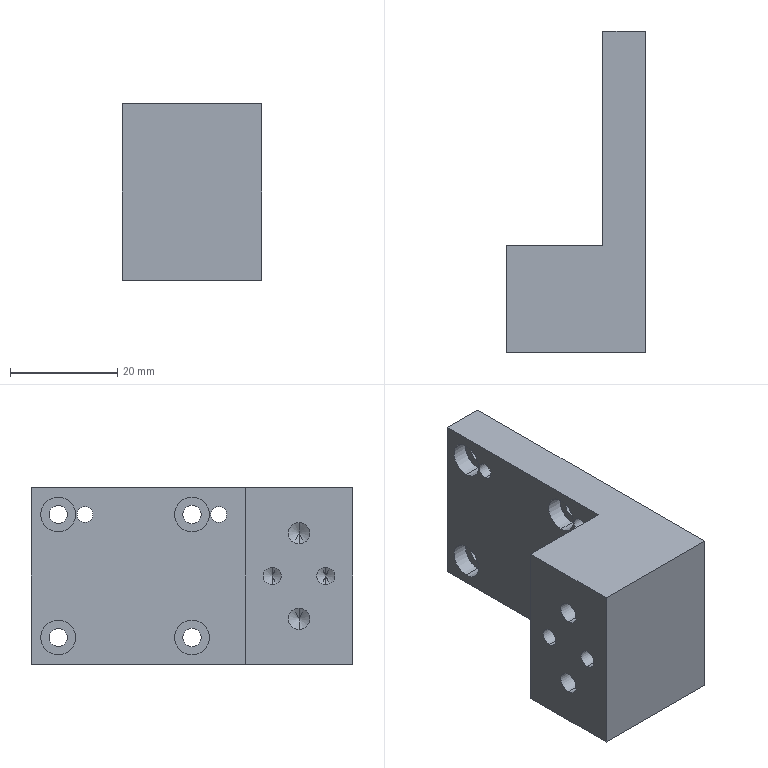Part | SolidWorks | features HoleWzd 4, LPattern 4, ICE 2, Extrusion 1 | 1 solid | 48 faces | box 26 x 60 x 33 mm | volume 26587 mm3 | cylinder 28 | plane 12 | cone 8 | commonest cylinder face diameters 3.4 x8 6.5 x8 3 x4 3.3 x4 4 x4
STEP:
#1=CARTESIAN_POINT('',(-8.,-20.,6.));
#2=VERTEX_POINT('',#1);
#3=CARTESIAN_POINT('',(-8.,-20.,10.));
#4=VERTEX_POINT('',#3);
#5=CARTESIAN_POINT('',(-8.,-20.,8.));
#6=DIRECTION('',(-1.,0.,0.));
#7=DIRECTION('',(0.,0.,1.));
#8=AXIS2_PLACEMENT_3D('',#5,#6,#7);
#9=CIRCLE('',#8,2.);
#10=EDGE_CURVE('',#2,#4,#9,.T.);
#11=ORIENTED_EDGE('',*,*,#10,.F.);
#12=CARTESIAN_POINT('',(-18.,-20.,6.));
#13=VERTEX_POINT('',#12);
#14=CARTESIAN_POINT('',(-18.,-20.,6.));
#15=DIRECTION('',(-1.,0.,0.));
#16=VECTOR('',#15,1000.);
#17=LINE('',#14,#16);
#18=EDGE_CURVE('',#2,#13,#17,.T.);
#19=ORIENTED_EDGE('',*,*,#18,.T.);
#20=CARTESIAN_POINT('',(-18.,-20.,10.));
#21=VERTEX_POINT('',#20);
#22=CARTESIAN_POINT('',(-18.,-20.,8.));
#23=DIRECTION('',(-1.,0.,0.));
#24=DIRECTION('',(0.,0.,1.));
#25=AXIS2_PLACEMENT_3D('',#22,#23,#24);
#26=CIRCLE('',#25,2.);
#27=EDGE_CURVE('',#13,#21,#26,.T.);
#28=ORIENTED_EDGE('',*,*,#27,.T.);
#29=CARTESIAN_POINT('',(-18.,-20.,10.));
#30=DIRECTION('',(-1.,0.,0.));
#31=VECTOR('',#30,1000.);
#32=LINE('',#29,#31);
#33=EDGE_CURVE('',#4,#21,#32,.T.);
#34=ORIENTED_EDGE('',*,*,#33,.F.);
#35=EDGE_LOOP('',(#11,#19,#28,#34));
#36=FACE_OUTER_BOUND('',#35,.T.);
#37=CARTESIAN_POINT('',(-18.,-20.,8.));
#38=DIRECTION('',(-1.,0.,0.));
#39=DIRECTION('',(0.,0.,1.));
#40=AXIS2_PLACEMENT_3D('',#37,#38,#39);
#41=CYLINDRICAL_SURFACE('',#40,2.);
#42=ADVANCED_FACE('',(#36),#41,.F.);
#43=CARTESIAN_POINT('',(-6.798,-20.,8.));
#44=VERTEX_POINT('',#43);
#45=CARTESIAN_POINT('',(-8.,-20.,10.));
#46=DIRECTION('',(-0.515,0.,0.8572));
#47=VECTOR('',#46,1000.);
#48=LINE('',#45,#47);
#49=EDGE_CURVE('',#44,#4,#48,.T.);
#50=ORIENTED_EDGE('',*,*,#49,.F.);
#51=CARTESIAN_POINT('',(-8.,-20.,6.));
#52=DIRECTION('',(-0.515,0.,-0.8572));
#53=VECTOR('',#52,1000.);
#54=LINE('',#51,#53);
#55=EDGE_CURVE('',#44,#2,#54,.T.);
#56=ORIENTED_EDGE('',*,*,#55,.T.);
#57=ORIENTED_EDGE('',*,*,#10,.T.);
#58=EDGE_LOOP('',(#50,#56,#57));
#59=FACE_OUTER_BOUND('',#58,.T.);
#60=CARTESIAN_POINT('',(-8.,-20.,8.));
#61=DIRECTION('',(-1.,0.,0.));
#62=DIRECTION('',(0.,0.,1.));
#63=AXIS2_PLACEMENT_3D('',#60,#61,#62);
#64=CONICAL_SURFACE('',#63,2.,1.03);
#65=ADVANCED_FACE('',(#59),#64,.F.);
#66=CARTESIAN_POINT('',(-8.,-20.,-10.));
#67=VERTEX_POINT('',#66);
#68=CARTESIAN_POINT('',(-8.,-20.,-6.));
#69=VERTEX_POINT('',#68);
#70=CARTESIAN_POINT('',(-8.,-20.,-8.));
#71=DIRECTION('',(-1.,0.,0.));
#72=DIRECTION('',(0.,0.,1.));
#73=AXIS2_PLACEMENT_3D('',#70,#71,#72);
#74=CIRCLE('',#73,2.);
#75=EDGE_CURVE('',#67,#69,#74,.T.);
#76=ORIENTED_EDGE('',*,*,#75,.F.);
#77=CARTESIAN_POINT('',(-18.,-20.,-10.));
#78=VERTEX_POINT('',#77);
#79=CARTESIAN_POINT('',(-18.,-20.,-10.));
#80=DIRECTION('',(-1.,0.,0.));
#81=VECTOR('',#80,1000.);
#82=LINE('',#79,#81);
#83=EDGE_CURVE('',#67,#78,#82,.T.);
#84=ORIENTED_EDGE('',*,*,#83,.T.);
#85=CARTESIAN_POINT('',(-18.,-20.,-6.));
#86=VERTEX_POINT('',#85);
#87=CARTESIAN_POINT('',(-18.,-20.,-8.));
#88=DIRECTION('',(-1.,0.,0.));
#89=DIRECTION('',(0.,0.,1.));
#90=AXIS2_PLACEMENT_3D('',#87,#88,#89);
#91=CIRCLE('',#90,2.);
#92=EDGE_CURVE('',#78,#86,#91,.T.);
#93=ORIENTED_EDGE('',*,*,#92,.T.);
#94=CARTESIAN_POINT('',(-18.,-20.,-6.));
#95=DIRECTION('',(-1.,0.,0.));
#96=VECTOR('',#95,1000.);
#97=LINE('',#94,#96);
#98=EDGE_CURVE('',#69,#86,#97,.T.);
#99=ORIENTED_EDGE('',*,*,#98,.F.);
#100=EDGE_LOOP('',(#76,#84,#93,#99));
#101=FACE_OUTER_BOUND('',#100,.T.);
#102=CARTESIAN_POINT('',(-18.,-20.,-8.));
#103=DIRECTION('',(-1.,0.,0.));
#104=DIRECTION('',(0.,0.,1.));
#105=AXIS2_PLACEMENT_3D('',#102,#103,#104);
#106=CYLINDRICAL_SURFACE('',#105,2.);
#107=ADVANCED_FACE('',(#101),#106,.F.);
#108=CARTESIAN_POINT('',(-6.798,-20.,-8.));
#109=VERTEX_POINT('',#108);
#110=CARTESIAN_POINT('',(-8.,-20.,-6.));
#111=DIRECTION('',(-0.515,0.,0.8572));
#112=VECTOR('',#111,1000.);
#113=LINE('',#110,#112);
#114=EDGE_CURVE('',#109,#69,#113,.T.);
#115=ORIENTED_EDGE('',*,*,#114,.F.);
#116=CARTESIAN_POINT('',(-8.,-20.,-10.));
#117=DIRECTION('',(-0.515,0.,-0.8572));
#118=VECTOR('',#117,1000.);
#119=LINE('',#116,#118);
#120=EDGE_CURVE('',#109,#67,#119,.T.);
#121=ORIENTED_EDGE('',*,*,#120,.T.);
#122=ORIENTED_EDGE('',*,*,#75,.T.);
#123=EDGE_LOOP('',(#115,#121,#122));
#124=FACE_OUTER_BOUND('',#123,.T.);
#125=CARTESIAN_POINT('',(-8.,-20.,-8.));
#126=DIRECTION('',(-1.,0.,0.));
#127=DIRECTION('',(0.,0.,1.));
#128=AXIS2_PLACEMENT_3D('',#125,#126,#127);
#129=CONICAL_SURFACE('',#128,2.,1.03);
#130=ADVANCED_FACE('',(#124),#129,.F.);
#131=CARTESIAN_POINT('',(8.,-5.,10.));
#132=VERTEX_POINT('',#131);
#133=CARTESIAN_POINT('',(8.,-5.,13.));
#134=VERTEX_POINT('',#133);
#135=CARTESIAN_POINT('',(8.,-5.,11.5));
#136=DIRECTION('',(-1.,0.,0.));
#137=DIRECTION('',(0.,0.,1.));
#138=AXIS2_PLACEMENT_3D('',#135,#136,#137);
#139=CIRCLE('',#138,1.5);
#140=EDGE_CURVE('',#132,#134,#139,.T.);
#141=ORIENTED_EDGE('',*,*,#140,.F.);
#142=CARTESIAN_POINT('',(0.,-5.,10.));
#143=VERTEX_POINT('',#142);
#144=CARTESIAN_POINT('',(0.,-5.,10.));
#145=DIRECTION('',(-1.,0.,0.));
#146=VECTOR('',#145,1000.);
#147=LINE('',#144,#146);
#148=EDGE_CURVE('',#132,#143,#147,.T.);
#149=ORIENTED_EDGE('',*,*,#148,.T.);
#150=CARTESIAN_POINT('',(0.,-5.,13.));
#151=VERTEX_POINT('',#150);
#152=CARTESIAN_POINT('',(0.,-5.,11.5));
#153=DIRECTION('',(-1.,0.,0.));
#154=DIRECTION('',(0.,0.,1.));
#155=AXIS2_PLACEMENT_3D('',#152,#153,#154);
#156=CIRCLE('',#155,1.5);
#157=EDGE_CURVE('',#143,#151,#156,.T.);
#158=ORIENTED_EDGE('',*,*,#157,.T.);
#159=CARTESIAN_POINT('',(0.,-5.,13.));
#160=DIRECTION('',(-1.,0.,0.));
#161=VECTOR('',#160,1000.);
#162=LINE('',#159,#161);
#163=EDGE_CURVE('',#134,#151,#162,.T.);
#164=ORIENTED_EDGE('',*,*,#163,.F.);
#165=EDGE_LOOP('',(#141,#149,#158,#164));
#166=FACE_OUTER_BOUND('',#165,.T.);
#167=CARTESIAN_POINT('',(0.,-5.,11.5));
#168=DIRECTION('',(-1.,0.,0.));
#169=DIRECTION('',(0.,0.,1.));
#170=AXIS2_PLACEMENT_3D('',#167,#168,#169);
#171=CYLINDRICAL_SURFACE('',#170,1.5);
#172=ADVANCED_FACE('',(#166),#171,.F.);
#173=CARTESIAN_POINT('',(8.,20.,10.));
#174=VERTEX_POINT('',#173);
#175=CARTESIAN_POINT('',(8.,20.,13.));
#176=VERTEX_POINT('',#175);
#177=CARTESIAN_POINT('',(8.,20.,11.5));
#178=DIRECTION('',(-1.,0.,0.));
#179=DIRECTION('',(0.,0.,1.));
#180=AXIS2_PLACEMENT_3D('',#177,#178,#179);
#181=CIRCLE('',#180,1.5);
#182=EDGE_CURVE('',#174,#176,#181,.T.);
#183=ORIENTED_EDGE('',*,*,#182,.F.);
#184=CARTESIAN_POINT('',(0.,20.,10.));
#185=VERTEX_POINT('',#184);
#186=CARTESIAN_POINT('',(0.,20.,10.));
#187=DIRECTION('',(-1.,0.,0.));
#188=VECTOR('',#187,1000.);
#189=LINE('',#186,#188);
#190=EDGE_CURVE('',#174,#185,#189,.T.);
#191=ORIENTED_EDGE('',*,*,#190,.T.);
#192=CARTESIAN_POINT('',(0.,20.,13.));
#193=VERTEX_POINT('',#192);
#194=CARTESIAN_POINT('',(0.,20.,11.5));
#195=DIRECTION('',(-1.,0.,0.));
#196=DIRECTION('',(0.,0.,1.));
#197=AXIS2_PLACEMENT_3D('',#194,#195,#196);
#198=CIRCLE('',#197,1.5);
#199=EDGE_CURVE('',#185,#193,#198,.T.);
#200=ORIENTED_EDGE('',*,*,#199,.T.);
#201=CARTESIAN_POINT('',(0.,20.,13.));
#202=DIRECTION('',(-1.,0.,0.));
#203=VECTOR('',#202,1000.);
#204=LINE('',#201,#203);
#205=EDGE_CURVE('',#176,#193,#204,.T.);
#206=ORIENTED_EDGE('',*,*,#205,.F.);
#207=EDGE_LOOP('',(#183,#191,#200,#206));
#208=FACE_OUTER_BOUND('',#207,.T.);
#209=CARTESIAN_POINT('',(0.,20.,11.5));
#210=DIRECTION('',(-1.,0.,0.));
#211=DIRECTION('',(0.,0.,1.));
#212=AXIS2_PLACEMENT_3D('',#209,#210,#211);
#213=CYLINDRICAL_SURFACE('',#212,1.5);
#214=ADVANCED_FACE('',(#208),#213,.F.);
#215=CARTESIAN_POINT('',(-7.9,-15.,-1.65));
#216=VERTEX_POINT('',#215);
#217=CARTESIAN_POINT('',(-7.9,-15.,1.65));
#218=VERTEX_POINT('',#217);
#219=CARTESIAN_POINT('',(-7.9,-15.,0.));
#220=DIRECTION('',(-1.,0.,0.));
#221=DIRECTION('',(0.,0.,1.));
#222=AXIS2_PLACEMENT_3D('',#219,#220,#221);
#223=CIRCLE('',#222,1.65);
#224=EDGE_CURVE('',#216,#218,#223,.T.);
#225=ORIENTED_EDGE('',*,*,#224,.F.);
#226=CARTESIAN_POINT('',(-18.,-15.,-1.65));
#227=VERTEX_POINT('',#226);
#228=CARTESIAN_POINT('',(-18.,-15.,-1.65));
#229=DIRECTION('',(-1.,0.,0.));
#230=VECTOR('',#229,1000.);
#231=LINE('',#228,#230);
#232=EDGE_CURVE('',#216,#227,#231,.T.);
#233=ORIENTED_EDGE('',*,*,#232,.T.);
#234=CARTESIAN_POINT('',(-18.,-15.,1.65));
#235=VERTEX_POINT('',#234);
#236=CARTESIAN_POINT('',(-18.,-15.,0.));
#237=DIRECTION('',(-1.,0.,0.));
#238=DIRECTION('',(0.,0.,1.));
#239=AXIS2_PLACEMENT_3D('',#236,#237,#238);
#240=CIRCLE('',#239,1.65);
#241=EDGE_CURVE('',#227,#235,#240,.T.);
#242=ORIENTED_EDGE('',*,*,#241,.T.);
#243=CARTESIAN_POINT('',(-18.,-15.,1.65));
#244=DIRECTION('',(-1.,0.,0.));
#245=VECTOR('',#244,1000.);
#246=LINE('',#243,#245);
#247=EDGE_CURVE('',#218,#235,#246,.T.);
#248=ORIENTED_EDGE('',*,*,#247,.F.);
#249=EDGE_LOOP('',(#225,#233,#242,#248));
#250=FACE_OUTER_BOUND('',#249,.T.);
#251=CARTESIAN_POINT('',(-18.,-15.,0.));
#252=DIRECTION('',(-1.,0.,0.));
#253=DIRECTION('',(0.,0.,1.));
#254=AXIS2_PLACEMENT_3D('',#251,#252,#253);
#255=CYLINDRICAL_SURFACE('',#254,1.65);
#256=ADVANCED_FACE('',(#250),#255,.F.);
#257=CARTESIAN_POINT('',(-6.909,-15.,0.));
#258=VERTEX_POINT('',#257);
#259=CARTESIAN_POINT('',(-7.9,-15.,1.65));
#260=DIRECTION('',(-0.515,0.,0.8572));
#261=VECTOR('',#260,1000.);
#262=LINE('',#259,#261);
#263=EDGE_CURVE('',#258,#218,#262,.T.);
#264=ORIENTED_EDGE('',*,*,#263,.F.);
#265=CARTESIAN_POINT('',(-7.9,-15.,-1.65));
#266=DIRECTION('',(-0.515,0.,-0.8572));
#267=VECTOR('',#266,1000.);
#268=LINE('',#265,#267);
#269=EDGE_CURVE('',#258,#216,#268,.T.);
#270=ORIENTED_EDGE('',*,*,#269,.T.);
#271=ORIENTED_EDGE('',*,*,#224,.T.);
#272=EDGE_LOOP('',(#264,#270,#271));
#273=FACE_OUTER_BOUND('',#272,.T.);
#274=CARTESIAN_POINT('',(-7.9,-15.,0.));
#275=DIRECTION('',(-1.,0.,0.));
#276=DIRECTION('',(0.,0.,1.));
#277=AXIS2_PLACEMENT_3D('',#274,#275,#276);
#278=CONICAL_SURFACE('',#277,1.65,1.03);
#279=ADVANCED_FACE('',(#273),#278,.F.);
#280=CARTESIAN_POINT('',(-7.9,-25.,-1.65));
#281=VERTEX_POINT('',#280);
#282=CARTESIAN_POINT('',(-7.9,-25.,1.65));
#283=VERTEX_POINT('',#282);
#284=CARTESIAN_POINT('',(-7.9,-25.,0.));
#285=DIRECTION('',(-1.,0.,0.));
#286=DIRECTION('',(0.,0.,1.));
#287=AXIS2_PLACEMENT_3D('',#284,#285,#286);
#288=CIRCLE('',#287,1.65);
#289=EDGE_CURVE('',#281,#283,#288,.T.);
#290=ORIENTED_EDGE('',*,*,#289,.F.);
#291=CARTESIAN_POINT('',(-18.,-25.,-1.65));
#292=VERTEX_POINT('',#291);
#293=CARTESIAN_POINT('',(-18.,-25.,-1.65));
#294=DIRECTION('',(-1.,0.,0.));
#295=VECTOR('',#294,1000.);
#296=LINE('',#293,#295);
#297=EDGE_CURVE('',#281,#292,#296,.T.);
#298=ORIENTED_EDGE('',*,*,#297,.T.);
#299=CARTESIAN_POINT('',(-18.,-25.,1.65));
#300=VERTEX_POINT('',#299);
#301=CARTESIAN_POINT('',(-18.,-25.,0.));
#302=DIRECTION('',(-1.,0.,0.));
#303=DIRECTION('',(0.,0.,1.));
#304=AXIS2_PLACEMENT_3D('',#301,#302,#303);
#305=CIRCLE('',#304,1.65);
#306=EDGE_CURVE('',#292,#300,#305,.T.);
#307=ORIENTED_EDGE('',*,*,#306,.T.);
#308=CARTESIAN_POINT('',(-18.,-25.,1.65));
#309=DIRECTION('',(-1.,0.,0.));
#310=VECTOR('',#309,1000.);
#311=LINE('',#308,#310);
#312=EDGE_CURVE('',#283,#300,#311,.T.);
#313=ORIENTED_EDGE('',*,*,#312,.F.);
#314=EDGE_LOOP('',(#290,#298,#307,#313));
#315=FACE_OUTER_BOUND('',#314,.T.);
#316=CARTESIAN_POINT('',(-18.,-25.,0.));
#317=DIRECTION('',(-1.,0.,0.));
#318=DIRECTION('',(0.,0.,1.));
#319=AXIS2_PLACEMENT_3D('',#316,#317,#318);
#320=CYLINDRICAL_SURFACE('',#319,1.65);
#321=ADVANCED_FACE('',(#315),#320,.F.);
#322=CARTESIAN_POINT('',(-6.909,-25.,0.));
#323=VERTEX_POINT('',#322);
#324=CARTESIAN_POINT('',(-7.9,-25.,1.65));
#325=DIRECTION('',(-0.515,0.,0.8572));
#326=VECTOR('',#325,1000.);
#327=LINE('',#324,#326);
#328=EDGE_CURVE('',#323,#283,#327,.T.);
#329=ORIENTED_EDGE('',*,*,#328,.F.);
#330=CARTESIAN_POINT('',(-7.9,-25.,-1.65));
#331=DIRECTION('',(-0.515,0.,-0.8572));
#332=VECTOR('',#331,1000.);
#333=LINE('',#330,#332);
#334=EDGE_CURVE('',#323,#281,#333,.T.);
#335=ORIENTED_EDGE('',*,*,#334,.T.);
#336=ORIENTED_EDGE('',*,*,#289,.T.);
#337=EDGE_LOOP('',(#329,#335,#336));
#338=FACE_OUTER_BOUND('',#337,.T.);
#339=CARTESIAN_POINT('',(-7.9,-25.,0.));
#340=DIRECTION('',(-1.,0.,0.));
#341=DIRECTION('',(0.,0.,1.));
#342=AXIS2_PLACEMENT_3D('',#339,#340,#341);
#343=CONICAL_SURFACE('',#342,1.65,1.03);
#344=ADVANCED_FACE('',(#338),#343,.F.);
#345=CARTESIAN_POINT('',(8.,0.,9.8));
#346=VERTEX_POINT('',#345);
#347=CARTESIAN_POINT('',(8.,0.,13.2));
#348=VERTEX_POINT('',#347);
#349=CARTESIAN_POINT('',(8.,0.,11.5));
#350=DIRECTION('',(-1.,0.,0.));
#351=DIRECTION('',(0.,0.,1.));
#352=AXIS2_PLACEMENT_3D('',#349,#350,#351);
#353=CIRCLE('',#352,1.7);
#354=EDGE_CURVE('',#346,#348,#353,.T.);
#355=ORIENTED_EDGE('',*,*,#354,.F.);
#356=CARTESIAN_POINT('',(3.,0.,9.8));
#357=VERTEX_POINT('',#356);
#358=CARTESIAN_POINT('',(0.,0.,9.8));
#359=DIRECTION('',(-1.,0.,0.));
#360=VECTOR('',#359,1000.);
#361=LINE('',#358,#360);
#362=EDGE_CURVE('',#346,#357,#361,.T.);
#363=ORIENTED_EDGE('',*,*,#362,.T.);
#364=CARTESIAN_POINT('',(3.,0.,13.2));
#365=VERTEX_POINT('',#364);
#366=CARTESIAN_POINT('',(3.,0.,11.5));
#367=DIRECTION('',(-1.,0.,0.));
#368=DIRECTION('',(0.,0.,1.));
#369=AXIS2_PLACEMENT_3D('',#366,#367,#368);
#370=CIRCLE('',#369,1.7);
#371=EDGE_CURVE('',#357,#365,#370,.T.);
#372=ORIENTED_EDGE('',*,*,#371,.T.);
#373=CARTESIAN_POINT('',(0.,0.,13.2));
#374=DIRECTION('',(-1.,0.,0.));
#375=VECTOR('',#374,1000.);
#376=LINE('',#373,#375);
#377=EDGE_CURVE('',#348,#365,#376,.T.);
#378=ORIENTED_EDGE('',*,*,#377,.F.);
#379=EDGE_LOOP('',(#355,#363,#372,#378));
#380=FACE_OUTER_BOUND('',#379,.T.);
#381=CARTESIAN_POINT('',(0.,0.,11.5));
#382=DIRECTION('',(-1.,0.,0.));
#383=DIRECTION('',(0.,0.,1.));
#384=AXIS2_PLACEMENT_3D('',#381,#382,#383);
#385=CYLINDRICAL_SURFACE('',#384,1.7);
#386=ADVANCED_FACE('',(#380),#385,.F.);
#387=CARTESIAN_POINT('',(3.,0.,8.25));
#388=VERTEX_POINT('',#387);
#389=CARTESIAN_POINT('',(3.,0.,14.75));
#390=VERTEX_POINT('',#389);
#391=CARTESIAN_POINT('',(3.,0.,11.5));
#392=DIRECTION('',(-1.,0.,0.));
#393=DIRECTION('',(0.,0.,1.));
#394=AXIS2_PLACEMENT_3D('',#391,#392,#393);
#395=CIRCLE('',#394,3.25);
#396=EDGE_CURVE('',#388,#390,#395,.T.);
#397=ORIENTED_EDGE('',*,*,#396,.F.);
#398=CARTESIAN_POINT('',(0.,0.,8.25));
#399=VERTEX_POINT('',#398);
#400=CARTESIAN_POINT('',(0.,0.,8.25));
#401=DIRECTION('',(-1.,0.,0.));
#402=VECTOR('',#401,1000.);
#403=LINE('',#400,#402);
#404=EDGE_CURVE('',#388,#399,#403,.T.);
#405=ORIENTED_EDGE('',*,*,#404,.T.);
#406=CARTESIAN_POINT('',(0.,0.,14.75));
#407=VERTEX_POINT('',#406);
#408=CARTESIAN_POINT('',(0.,0.,11.5));
#409=DIRECTION('',(-1.,0.,0.));
#410=DIRECTION('',(0.,0.,1.));
#411=AXIS2_PLACEMENT_3D('',#408,#409,#410);
#412=CIRCLE('',#411,3.25);
#413=EDGE_CURVE('',#399,#407,#412,.T.);
#414=ORIENTED_EDGE('',*,*,#413,.T.);
#415=CARTESIAN_POINT('',(0.,0.,14.75));
#416=DIRECTION('',(-1.,0.,0.));
#417=VECTOR('',#416,1000.);
#418=LINE('',#415,#417);
#419=EDGE_CURVE('',#390,#407,#418,.T.);
#420=ORIENTED_EDGE('',*,*,#419,.F.);
#421=EDGE_LOOP('',(#397,#405,#414,#420));
#422=FACE_OUTER_BOUND('',#421,.T.);
#423=CARTESIAN_POINT('',(0.,0.,11.5));
#424=DIRECTION('',(-1.,0.,0.));
#425=DIRECTION('',(0.,0.,1.));
#426=AXIS2_PLACEMENT_3D('',#423,#424,#425);
#427=CYLINDRICAL_SURFACE('',#426,3.25);
#428=ADVANCED_FACE('',(#422),#427,.F.);
#429=CARTESIAN_POINT('',(8.,0.,-13.2));
#430=VERTEX_POINT('',#429);
#431=CARTESIAN_POINT('',(8.,0.,-9.8));
#432=VERTEX_POINT('',#431);
#433=CARTESIAN_POINT('',(8.,0.,-11.5));
#434=DIRECTION('',(-1.,0.,0.));
#435=DIRECTION('',(0.,0.,1.));
#436=AXIS2_PLACEMENT_3D('',#433,#434,#435);
#437=CIRCLE('',#436,1.7);
#438=EDGE_CURVE('',#430,#432,#437,.T.);
#439=ORIENTED_EDGE('',*,*,#438,.F.);
#440=CARTESIAN_POINT('',(3.,0.,-13.2));
#441=VERTEX_POINT('',#440);
#442=CARTESIAN_POINT('',(0.,0.,-13.2));
#443=DIRECTION('',(-1.,0.,0.));
#444=VECTOR('',#443,1000.);
#445=LINE('',#442,#444);
#446=EDGE_CURVE('',#430,#441,#445,.T.);
#447=ORIENTED_EDGE('',*,*,#446,.T.);
#448=CARTESIAN_POINT('',(3.,0.,-9.8));
#449=VERTEX_POINT('',#448);
#450=CARTESIAN_POINT('',(3.,0.,-11.5));
#451=DIRECTION('',(-1.,0.,0.));
#452=DIRECTION('',(0.,0.,1.));
#453=AXIS2_PLACEMENT_3D('',#450,#451,#452);
#454=CIRCLE('',#453,1.7);
#455=EDGE_CURVE('',#441,#449,#454,.T.);
#456=ORIENTED_EDGE('',*,*,#455,.T.);
#457=CARTESIAN_POINT('',(0.,0.,-9.8));
#458=DIRECTION('',(-1.,0.,0.));
#459=VECTOR('',#458,1000.);
#460=LINE('',#457,#459);
#461=EDGE_CURVE('',#432,#449,#460,.T.);
#462=ORIENTED_EDGE('',*,*,#461,.F.);
#463=EDGE_LOOP('',(#439,#447,#456,#462));
#464=FACE_OUTER_BOUND('',#463,.T.);
#465=CARTESIAN_POINT('',(0.,0.,-11.5));
#466=DIRECTION('',(-1.,0.,0.));
#467=DIRECTION('',(0.,0.,1.));
#468=AXIS2_PLACEMENT_3D('',#465,#466,#467);
#469=CYLINDRICAL_SURFACE('',#468,1.7);
#470=ADVANCED_FACE('',(#464),#469,.F.);
#471=CARTESIAN_POINT('',(3.,0.,-14.75));
#472=VERTEX_POINT('',#471);
#473=CARTESIAN_POINT('',(3.,0.,-8.25));
#474=VERTEX_POINT('',#473);
#475=CARTESIAN_POINT('',(3.,0.,-11.5));
#476=DIRECTION('',(-1.,0.,0.));
#477=DIRECTION('',(0.,0.,1.));
#478=AXIS2_PLACEMENT_3D('',#475,#476,#477);
#479=CIRCLE('',#478,3.25);
#480=EDGE_CURVE('',#472,#474,#479,.T.);
#481=ORIENTED_EDGE('',*,*,#480,.F.);
#482=CARTESIAN_POINT('',(0.,0.,-14.75));
#483=VERTEX_POINT('',#482);
#484=CARTESIAN_POINT('',(0.,0.,-14.75));
#485=DIRECTION('',(-1.,0.,0.));
#486=VECTOR('',#485,1000.);
#487=LINE('',#484,#486);
#488=EDGE_CURVE('',#472,#483,#487,.T.);
#489=ORIENTED_EDGE('',*,*,#488,.T.);
#490=CARTESIAN_POINT('',(0.,0.,-8.25));
#491=VERTEX_POINT('',#490);
#492=CARTESIAN_POINT('',(0.,0.,-11.5));
#493=DIRECTION('',(-1.,0.,0.));
#494=DIRECTION('',(0.,0.,1.));
#495=AXIS2_PLACEMENT_3D('',#492,#493,#494);
#496=CIRCLE('',#495,3.25);
#497=EDGE_CURVE('',#483,#491,#496,.T.);
#498=ORIENTED_EDGE('',*,*,#497,.T.);
#499=CARTESIAN_POINT('',(0.,0.,-8.25));
#500=DIRECTION('',(-1.,0.,0.));
#501=VECTOR('',#500,1000.);
#502=LINE('',#499,#501);
#503=EDGE_CURVE('',#474,#491,#502,.T.);
#504=ORIENTED_EDGE('',*,*,#503,.F.);
#505=EDGE_LOOP('',(#481,#489,#498,#504));
#506=FACE_OUTER_BOUND('',#505,.T.);
#507=CARTESIAN_POINT('',(0.,0.,-11.5));
#508=DIRECTION('',(-1.,0.,0.));
#509=DIRECTION('',(0.,0.,1.));
#510=AXIS2_PLACEMENT_3D('',#507,#508,#509);
#511=CYLINDRICAL_SURFACE('',#510,3.25);
#512=ADVANCED_FACE('',(#506),#511,.F.);
#513=CARTESIAN_POINT('',(3.,25.,8.25));
#514=VERTEX_POINT('',#513);
#515=CARTESIAN_POINT('',(3.,25.,14.75));
#516=VERTEX_POINT('',#515);
#517=CARTESIAN_POINT('',(3.,25.,11.5));
#518=DIRECTION('',(-1.,0.,0.));
#519=DIRECTION('',(0.,0.,1.));
#520=AXIS2_PLACEMENT_3D('',#517,#518,#519);
#521=CIRCLE('',#520,3.25);
#522=EDGE_CURVE('',#514,#516,#521,.T.);
#523=ORIENTED_EDGE('',*,*,#522,.F.);
#524=CARTESIAN_POINT('',(0.,25.,8.25));
#525=VERTEX_POINT('',#524);
#526=CARTESIAN_POINT('',(0.,25.,8.25));
#527=DIRECTION('',(-1.,0.,0.));
#528=VECTOR('',#527,1000.);
#529=LINE('',#526,#528);
#530=EDGE_CURVE('',#514,#525,#529,.T.);
#531=ORIENTED_EDGE('',*,*,#530,.T.);
#532=CARTESIAN_POINT('',(0.,25.,14.75));
#533=VERTEX_POINT('',#532);
#534=CARTESIAN_POINT('',(0.,25.,11.5));
#535=DIRECTION('',(-1.,0.,0.));
#536=DIRECTION('',(0.,0.,1.));
#537=AXIS2_PLACEMENT_3D('',#534,#535,#536);
#538=CIRCLE('',#537,3.25);
#539=EDGE_CURVE('',#525,#533,#538,.T.);
#540=ORIENTED_EDGE('',*,*,#539,.T.);
#541=CARTESIAN_POINT('',(0.,25.,14.75));
#542=DIRECTION('',(-1.,0.,0.));
#543=VECTOR('',#542,1000.);
#544=LINE('',#541,#543);
#545=EDGE_CURVE('',#516,#533,#544,.T.);
#546=ORIENTED_EDGE('',*,*,#545,.F.);
#547=EDGE_LOOP('',(#523,#531,#540,#546));
#548=FACE_OUTER_BOUND('',#547,.T.);
#549=CARTESIAN_POINT('',(0.,25.,11.5));
#550=DIRECTION('',(-1.,0.,0.));
#551=DIRECTION('',(0.,0.,1.));
#552=AXIS2_PLACEMENT_3D('',#549,#550,#551);
#553=CYLINDRICAL_SURFACE('',#552,3.25);
#554=ADVANCED_FACE('',(#548),#553,.F.);
#555=CARTESIAN_POINT('',(8.,25.,9.8));
#556=VERTEX_POINT('',#555);
#557=CARTESIAN_POINT('',(8.,25.,13.2));
#558=VERTEX_POINT('',#557);
#559=CARTESIAN_POINT('',(8.,25.,11.5));
#560=DIRECTION('',(-1.,0.,0.));
#561=DIRECTION('',(0.,0.,1.));
#562=AXIS2_PLACEMENT_3D('',#559,#560,#561);
#563=CIRCLE('',#562,1.7);
#564=EDGE_CURVE('',#556,#558,#563,.T.);
#565=ORIENTED_EDGE('',*,*,#564,.F.);
#566=CARTESIAN_POINT('',(3.,25.,9.8));
#567=VERTEX_POINT('',#566);
#568=CARTESIAN_POINT('',(0.,25.,9.8));
#569=DIRECTION('',(-1.,0.,0.));
#570=VECTOR('',#569,1000.);
#571=LINE('',#568,#570);
#572=EDGE_CURVE('',#556,#567,#571,.T.);
#573=ORIENTED_EDGE('',*,*,#572,.T.);
#574=CARTESIAN_POINT('',(3.,25.,13.2));
#575=VERTEX_POINT('',#574);
#576=CARTESIAN_POINT('',(3.,25.,11.5));
#577=DIRECTION('',(-1.,0.,0.));
#578=DIRECTION('',(0.,0.,1.));
#579=AXIS2_PLACEMENT_3D('',#576,#577,#578);
#580=CIRCLE('',#579,1.7);
#581=EDGE_CURVE('',#567,#575,#580,.T.);
#582=ORIENTED_EDGE('',*,*,#581,.T.);
#583=CARTESIAN_POINT('',(0.,25.,13.2));
#584=DIRECTION('',(-1.,0.,0.));
#585=VECTOR('',#584,1000.);
#586=LINE('',#583,#585);
#587=EDGE_CURVE('',#558,#575,#586,.T.);
#588=ORIENTED_EDGE('',*,*,#587,.F.);
#589=EDGE_LOOP('',(#565,#573,#582,#588));
#590=FACE_OUTER_BOUND('',#589,.T.);
#591=CARTESIAN_POINT('',(0.,25.,11.5));
#592=DIRECTION('',(-1.,0.,0.));
#593=DIRECTION('',(0.,0.,1.));
#594=AXIS2_PLACEMENT_3D('',#591,#592,#593);
#595=CYLINDRICAL_SURFACE('',#594,1.7);
#596=ADVANCED_FACE('',(#590),#595,.F.);
#597=CARTESIAN_POINT('',(3.,25.,-14.75));
#598=VERTEX_POINT('',#597);
#599=CARTESIAN_POINT('',(3.,25.,-8.25));
#600=VERTEX_POINT('',#599);
#601=CARTESIAN_POINT('',(3.,25.,-11.5));
#602=DIRECTION('',(-1.,0.,0.));
#603=DIRECTION('',(0.,0.,1.));
#604=AXIS2_PLACEMENT_3D('',#601,#602,#603);
#605=CIRCLE('',#604,3.25);
#606=EDGE_CURVE('',#598,#600,#605,.T.);
#607=ORIENTED_EDGE('',*,*,#606,.F.);
#608=CARTESIAN_POINT('',(0.,25.,-14.75));
#609=VERTEX_POINT('',#608);
#610=CARTESIAN_POINT('',(0.,25.,-14.75));
#611=DIRECTION('',(-1.,0.,0.));
#612=VECTOR('',#611,1000.);
#613=LINE('',#610,#612);
#614=EDGE_CURVE('',#598,#609,#613,.T.);
#615=ORIENTED_EDGE('',*,*,#614,.T.);
#616=CARTESIAN_POINT('',(0.,25.,-8.25));
#617=VERTEX_POINT('',#616);
#618=CARTESIAN_POINT('',(0.,25.,-11.5));
#619=DIRECTION('',(-1.,0.,0.));
#620=DIRECTION('',(0.,0.,1.));
#621=AXIS2_PLACEMENT_3D('',#618,#619,#620);
#622=CIRCLE('',#621,3.25);
#623=EDGE_CURVE('',#609,#617,#622,.T.);
#624=ORIENTED_EDGE('',*,*,#623,.T.);
#625=CARTESIAN_POINT('',(0.,25.,-8.25));
#626=DIRECTION('',(-1.,0.,0.));
#627=VECTOR('',#626,1000.);
#628=LINE('',#625,#627);
#629=EDGE_CURVE('',#600,#617,#628,.T.);
#630=ORIENTED_EDGE('',*,*,#629,.F.);
#631=EDGE_LOOP('',(#607,#615,#624,#630));
#632=FACE_OUTER_BOUND('',#631,.T.);
#633=CARTESIAN_POINT('',(0.,25.,-11.5));
#634=DIRECTION('',(-1.,0.,0.));
#635=DIRECTION('',(0.,0.,1.));
#636=AXIS2_PLACEMENT_3D('',#633,#634,#635);
#637=CYLINDRICAL_SURFACE('',#636,3.25);
#638=ADVANCED_FACE('',(#632),#637,.F.);
#639=CARTESIAN_POINT('',(8.,25.,-13.2));
#640=VERTEX_POINT('',#639);
#641=CARTESIAN_POINT('',(8.,25.,-9.8));
#642=VERTEX_POINT('',#641);
#643=CARTESIAN_POINT('',(8.,25.,-11.5));
#644=DIRECTION('',(-1.,0.,0.));
#645=DIRECTION('',(0.,0.,1.));
#646=AXIS2_PLACEMENT_3D('',#643,#644,#645);
#647=CIRCLE('',#646,1.7);
#648=EDGE_CURVE('',#640,#642,#647,.T.);
#649=ORIENTED_EDGE('',*,*,#648,.F.);
#650=CARTESIAN_POINT('',(3.,25.,-13.2));
#651=VERTEX_POINT('',#650);
#652=CARTESIAN_POINT('',(0.,25.,-13.2));
#653=DIRECTION('',(-1.,0.,0.));
#654=VECTOR('',#653,1000.);
#655=LINE('',#652,#654);
#656=EDGE_CURVE('',#640,#651,#655,.T.);
#657=ORIENTED_EDGE('',*,*,#656,.T.);
#658=CARTESIAN_POINT('',(3.,25.,-9.8));
#659=VERTEX_POINT('',#658);
#660=CARTESIAN_POINT('',(3.,25.,-11.5));
#661=DIRECTION('',(-1.,0.,0.));
#662=DIRECTION('',(0.,0.,1.));
#663=AXIS2_PLACEMENT_3D('',#660,#661,#662);
#664=CIRCLE('',#663,1.7);
#665=EDGE_CURVE('',#651,#659,#664,.T.);
#666=ORIENTED_EDGE('',*,*,#665,.T.);
#667=CARTESIAN_POINT('',(0.,25.,-9.8));
#668=DIRECTION('',(-1.,0.,0.));
#669=VECTOR('',#668,1000.);
#670=LINE('',#667,#669);
#671=EDGE_CURVE('',#642,#659,#670,.T.);
#672=ORIENTED_EDGE('',*,*,#671,.F.);
#673=EDGE_LOOP('',(#649,#657,#666,#672));
#674=FACE_OUTER_BOUND('',#673,.T.);
#675=CARTESIAN_POINT('',(0.,25.,-11.5));
#676=DIRECTION('',(-1.,0.,0.));
#677=DIRECTION('',(0.,0.,1.));
#678=AXIS2_PLACEMENT_3D('',#675,#676,#677);
#679=CYLINDRICAL_SURFACE('',#678,1.7);
#680=ADVANCED_FACE('',(#674),#679,.F.);
#681=CARTESIAN_POINT('',(-18.,-10.,-16.5));
#682=VERTEX_POINT('',#681);
#683=CARTESIAN_POINT('',(-18.,-30.,-16.5));
#684=VERTEX_POINT('',#683);
#685=CARTESIAN_POINT('',(-18.,-30.,-16.5));
#686=DIRECTION('',(0.,-1.,0.));
#687=VECTOR('',#686,1000.);
#688=LINE('',#685,#687);
#689=EDGE_CURVE('',#682,#684,#688,.T.);
#690=ORIENTED_EDGE('',*,*,#689,.F.);
#691=CARTESIAN_POINT('',(0.,-10.,-16.5));
#692=VERTEX_POINT('',#691);
#693=CARTESIAN_POINT('',(33.377,-10.,-16.5));
#694=DIRECTION('',(-1.,0.,0.));
#695=VECTOR('',#694,1000.);
#696=LINE('',#693,#695);
#697=EDGE_CURVE('',#692,#682,#696,.T.);
#698=ORIENTED_EDGE('',*,*,#697,.F.);
#699=CARTESIAN_POINT('',(0.,30.,-16.5));
#700=VERTEX_POINT('',#699);
#701=CARTESIAN_POINT('',(0.,-30.,-16.5));
#702=DIRECTION('',(0.,1.,0.));
#703=VECTOR('',#702,1000.);
#704=LINE('',#701,#703);
#705=EDGE_CURVE('',#692,#700,#704,.T.);
#706=ORIENTED_EDGE('',*,*,#705,.T.);
#707=CARTESIAN_POINT('',(8.,30.,-16.5));
#708=VERTEX_POINT('',#707);
#709=CARTESIAN_POINT('',(8.,30.,-16.5));
#710=DIRECTION('',(-1.,0.,0.));
#711=VECTOR('',#710,1000.);
#712=LINE('',#709,#711);
#713=EDGE_CURVE('',#708,#700,#712,.T.);
#714=ORIENTED_EDGE('',*,*,#713,.F.);
#715=CARTESIAN_POINT('',(8.,-30.,-16.5));
#716=VERTEX_POINT('',#715);
#717=CARTESIAN_POINT('',(8.,-30.,-16.5));
#718=DIRECTION('',(0.,1.,0.));
#719=VECTOR('',#718,1000.);
#720=LINE('',#717,#719);
#721=EDGE_CURVE('',#716,#708,#720,.T.);
#722=ORIENTED_EDGE('',*,*,#721,.F.);
#723=CARTESIAN_POINT('',(8.,-30.,-16.5));
#724=DIRECTION('',(-1.,0.,0.));
#725=VECTOR('',#724,1000.);
#726=LINE('',#723,#725);
#727=EDGE_CURVE('',#716,#684,#726,.T.);
#728=ORIENTED_EDGE('',*,*,#727,.T.);
#729=EDGE_LOOP('',(#690,#698,#706,#714,#722,#728));
#730=FACE_OUTER_BOUND('',#729,.T.);
#731=CARTESIAN_POINT('',(8.,-30.,-16.5));
#732=DIRECTION('',(0.,0.,1.));
#733=DIRECTION('',(1.,0.,0.));
#734=AXIS2_PLACEMENT_3D('',#731,#732,#733);
#735=PLANE('',#734);
#736=ADVANCED_FACE('',(#730),#735,.F.);
#737=CARTESIAN_POINT('',(0.,30.,16.5));
#738=VERTEX_POINT('',#737);
#739=CARTESIAN_POINT('',(0.,30.,16.5));
#740=DIRECTION('',(0.,0.,1.));
#741=VECTOR('',#740,1000.);
#742=LINE('',#739,#741);
#743=EDGE_CURVE('',#700,#738,#742,.T.);
#744=ORIENTED_EDGE('',*,*,#743,.T.);
#745=CARTESIAN_POINT('',(8.,30.,16.5));
#746=VERTEX_POINT('',#745);
#747=CARTESIAN_POINT('',(8.,30.,16.5));
#748=DIRECTION('',(-1.,0.,0.));
#749=VECTOR('',#748,1000.);
#750=LINE('',#747,#749);
#751=EDGE_CURVE('',#746,#738,#750,.T.);
#752=ORIENTED_EDGE('',*,*,#751,.F.);
#753=CARTESIAN_POINT('',(8.,30.,16.5));
#754=DIRECTION('',(0.,0.,1.));
#755=VECTOR('',#754,1000.);
#756=LINE('',#753,#755);
#757=EDGE_CURVE('',#708,#746,#756,.T.);
#758=ORIENTED_EDGE('',*,*,#757,.F.);
#759=ORIENTED_EDGE('',*,*,#713,.T.);
#760=EDGE_LOOP('',(#744,#752,#758,#759));
#761=FACE_OUTER_BOUND('',#760,.T.);
#762=CARTESIAN_POINT('',(8.,30.,16.5));
#763=DIRECTION('',(0.,-1.,0.));
#764=DIRECTION('',(0.,0.,-1.));
#765=AXIS2_PLACEMENT_3D('',#762,#763,#764);
#766=PLANE('',#765);
#767=ADVANCED_FACE('',(#761),#766,.F.);
#768=CARTESIAN_POINT('',(0.,-10.,16.5));
#769=VERTEX_POINT('',#768);
#770=CARTESIAN_POINT('',(0.,-30.,16.5));
#771=DIRECTION('',(0.,-1.,0.));
#772=VECTOR('',#771,1000.);
#773=LINE('',#770,#772);
#774=EDGE_CURVE('',#738,#769,#773,.T.);
#775=ORIENTED_EDGE('',*,*,#774,.T.);
#776=CARTESIAN_POINT('',(-18.,-10.,16.5));
#777=VERTEX_POINT('',#776);
#778=CARTESIAN_POINT('',(33.377,-10.,16.5));
#779=DIRECTION('',(-1.,0.,0.));
#780=VECTOR('',#779,1000.);
#781=LINE('',#778,#780);
#782=EDGE_CURVE('',#769,#777,#781,.T.);
#783=ORIENTED_EDGE('',*,*,#782,.T.);
#784=CARTESIAN_POINT('',(-18.,-30.,16.5));
#785=VERTEX_POINT('',#784);
#786=CARTESIAN_POINT('',(-18.,-30.,16.5));
#787=DIRECTION('',(0.,1.,0.));
#788=VECTOR('',#787,1000.);
#789=LINE('',#786,#788);
#790=EDGE_CURVE('',#785,#777,#789,.T.);
#791=ORIENTED_EDGE('',*,*,#790,.F.);
#792=CARTESIAN_POINT('',(8.,-30.,16.5));
#793=VERTEX_POINT('',#792);
#794=CARTESIAN_POINT('',(8.,-30.,16.5));
#795=DIRECTION('',(-1.,0.,0.));
#796=VECTOR('',#795,1000.);
#797=LINE('',#794,#796);
#798=EDGE_CURVE('',#793,#785,#797,.T.);
#799=ORIENTED_EDGE('',*,*,#798,.F.);
#800=CARTESIAN_POINT('',(8.,-30.,16.5));
#801=DIRECTION('',(0.,-1.,0.));
#802=VECTOR('',#801,1000.);
#803=LINE('',#800,#802);
#804=EDGE_CURVE('',#746,#793,#803,.T.);
#805=ORIENTED_EDGE('',*,*,#804,.F.);
#806=ORIENTED_EDGE('',*,*,#751,.T.);
#807=EDGE_LOOP('',(#775,#783,#791,#799,#805,#806));
#808=FACE_OUTER_BOUND('',#807,.T.);
#809=CARTESIAN_POINT('',(8.,-30.,16.5));
#810=DIRECTION('',(0.,0.,-1.));
#811=DIRECTION('',(-1.,0.,0.));
#812=AXIS2_PLACEMENT_3D('',#809,#810,#811);
#813=PLANE('',#812);
#814=ADVANCED_FACE('',(#808),#813,.F.);
#815=ORIENTED_EDGE('',*,*,#798,.T.);
#816=CARTESIAN_POINT('',(-18.,-30.,-16.5));
#817=DIRECTION('',(0.,0.,1.));
#818=VECTOR('',#817,1000.);
#819=LINE('',#816,#818);
#820=EDGE_CURVE('',#684,#785,#819,.T.);
#821=ORIENTED_EDGE('',*,*,#820,.F.);
#822=ORIENTED_EDGE('',*,*,#727,.F.);
#823=CARTESIAN_POINT('',(8.,-30.,16.5));
#824=DIRECTION('',(0.,0.,-1.));
#825=VECTOR('',#824,1000.);
#826=LINE('',#823,#825);
#827=EDGE_CURVE('',#793,#716,#826,.T.);
#828=ORIENTED_EDGE('',*,*,#827,.F.);
#829=EDGE_LOOP('',(#815,#821,#822,#828));
#830=FACE_OUTER_BOUND('',#829,.T.);
#831=CARTESIAN_POINT('',(8.,-30.,16.5));
#832=DIRECTION('',(0.,1.,0.));
#833=DIRECTION('',(0.,0.,1.));
#834=AXIS2_PLACEMENT_3D('',#831,#832,#833);
#835=PLANE('',#834);
#836=ADVANCED_FACE('',(#830),#835,.F.);
#837=CARTESIAN_POINT('',(8.,-5.,11.5));
#838=DIRECTION('',(-1.,0.,0.));
#839=DIRECTION('',(0.,0.,1.));
#840=AXIS2_PLACEMENT_3D('',#837,#838,#839);
#841=CIRCLE('',#840,1.5);
#842=EDGE_CURVE('',#134,#132,#841,.T.);
#843=ORIENTED_EDGE('',*,*,#842,.T.);
#844=ORIENTED_EDGE('',*,*,#140,.T.);
#845=EDGE_LOOP('',(#843,#844));
#846=FACE_BOUND('',#845,.T.);
#847=CARTESIAN_POINT('',(8.,20.,11.5));
#848=DIRECTION('',(-1.,0.,0.));
#849=DIRECTION('',(0.,0.,1.));
#850=AXIS2_PLACEMENT_3D('',#847,#848,#849);
#851=CIRCLE('',#850,1.5);
#852=EDGE_CURVE('',#176,#174,#851,.T.);
#853=ORIENTED_EDGE('',*,*,#852,.T.);
#854=ORIENTED_EDGE('',*,*,#182,.T.);
#855=EDGE_LOOP('',(#853,#854));
#856=FACE_BOUND('',#855,.T.);
#857=CARTESIAN_POINT('',(8.,25.,11.5));
#858=DIRECTION('',(-1.,0.,0.));
#859=DIRECTION('',(0.,0.,1.));
#860=AXIS2_PLACEMENT_3D('',#857,#858,#859);
#861=CIRCLE('',#860,1.7);
#862=EDGE_CURVE('',#558,#556,#861,.T.);
#863=ORIENTED_EDGE('',*,*,#862,.T.);
#864=ORIENTED_EDGE('',*,*,#564,.T.);
#865=EDGE_LOOP('',(#863,#864));
#866=FACE_BOUND('',#865,.T.);
#867=CARTESIAN_POINT('',(8.,25.,-11.5));
#868=DIRECTION('',(-1.,0.,0.));
#869=DIRECTION('',(0.,0.,1.));
#870=AXIS2_PLACEMENT_3D('',#867,#868,#869);
#871=CIRCLE('',#870,1.7);
#872=EDGE_CURVE('',#642,#640,#871,.T.);
#873=ORIENTED_EDGE('',*,*,#872,.T.);
#874=ORIENTED_EDGE('',*,*,#648,.T.);
#875=EDGE_LOOP('',(#873,#874));
#876=FACE_BOUND('',#875,.T.);
#877=ORIENTED_EDGE('',*,*,#721,.T.);
#878=ORIENTED_EDGE('',*,*,#757,.T.);
#879=ORIENTED_EDGE('',*,*,#804,.T.);
#880=ORIENTED_EDGE('',*,*,#827,.T.);
#881=EDGE_LOOP('',(#877,#878,#879,#880));
#882=FACE_OUTER_BOUND('',#881,.T.);
#883=CARTESIAN_POINT('',(8.,0.,-11.5));
#884=DIRECTION('',(-1.,0.,0.));
#885=DIRECTION('',(0.,0.,1.));
#886=AXIS2_PLACEMENT_3D('',#883,#884,#885);
#887=CIRCLE('',#886,1.7);
#888=EDGE_CURVE('',#432,#430,#887,.T.);
#889=ORIENTED_EDGE('',*,*,#888,.T.);
#890=ORIENTED_EDGE('',*,*,#438,.T.);
#891=EDGE_LOOP('',(#889,#890));
#892=FACE_BOUND('',#891,.T.);
#893=CARTESIAN_POINT('',(8.,0.,11.5));
#894=DIRECTION('',(-1.,0.,0.));
#895=DIRECTION('',(0.,0.,1.));
#896=AXIS2_PLACEMENT_3D('',#893,#894,#895);
#897=CIRCLE('',#896,1.7);
#898=EDGE_CURVE('',#348,#346,#897,.T.);
#899=ORIENTED_EDGE('',*,*,#898,.T.);
#900=ORIENTED_EDGE('',*,*,#354,.T.);
#901=EDGE_LOOP('',(#899,#900));
#902=FACE_BOUND('',#901,.T.);
#903=CARTESIAN_POINT('',(8.,30.,-16.5));
#904=DIRECTION('',(-1.,0.,0.));
#905=DIRECTION('',(0.,0.,1.));
#906=AXIS2_PLACEMENT_3D('',#903,#904,#905);
#907=PLANE('',#906);
#908=ADVANCED_FACE('',(#846,#856,#866,#876,#882,#892,#902),#907,.F.);
#909=CARTESIAN_POINT('',(0.,-5.,11.5));
#910=DIRECTION('',(-1.,0.,0.));
#911=DIRECTION('',(0.,0.,1.));
#912=AXIS2_PLACEMENT_3D('',#909,#910,#911);
#913=CIRCLE('',#912,1.5);
#914=EDGE_CURVE('',#151,#143,#913,.T.);
#915=ORIENTED_EDGE('',*,*,#914,.F.);
#916=ORIENTED_EDGE('',*,*,#157,.F.);
#917=EDGE_LOOP('',(#915,#916));
#918=FACE_BOUND('',#917,.T.);
#919=CARTESIAN_POINT('',(0.,20.,11.5));
#920=DIRECTION('',(-1.,0.,0.));
#921=DIRECTION('',(0.,0.,1.));
#922=AXIS2_PLACEMENT_3D('',#919,#920,#921);
#923=CIRCLE('',#922,1.5);
#924=EDGE_CURVE('',#193,#185,#923,.T.);
#925=ORIENTED_EDGE('',*,*,#924,.F.);
#926=ORIENTED_EDGE('',*,*,#199,.F.);
#927=EDGE_LOOP('',(#925,#926));
#928=FACE_BOUND('',#927,.T.);
#929=CARTESIAN_POINT('',(0.,25.,11.5));
#930=DIRECTION('',(-1.,0.,0.));
#931=DIRECTION('',(0.,0.,1.));
#932=AXIS2_PLACEMENT_3D('',#929,#930,#931);
#933=CIRCLE('',#932,3.25);
#934=EDGE_CURVE('',#533,#525,#933,.T.);
#935=ORIENTED_EDGE('',*,*,#934,.F.);
#936=ORIENTED_EDGE('',*,*,#539,.F.);
#937=EDGE_LOOP('',(#935,#936));
#938=FACE_BOUND('',#937,.T.);
#939=CARTESIAN_POINT('',(0.,25.,-11.5));
#940=DIRECTION('',(-1.,0.,0.));
#941=DIRECTION('',(0.,0.,1.));
#942=AXIS2_PLACEMENT_3D('',#939,#940,#941);
#943=CIRCLE('',#942,3.25);
#944=EDGE_CURVE('',#617,#609,#943,.T.);
#945=ORIENTED_EDGE('',*,*,#944,.F.);
#946=ORIENTED_EDGE('',*,*,#623,.F.);
#947=EDGE_LOOP('',(#945,#946));
#948=FACE_BOUND('',#947,.T.);
#949=ORIENTED_EDGE('',*,*,#705,.F.);
#950=CARTESIAN_POINT('',(0.,-10.,-16.5));
#951=DIRECTION('',(0.,0.,-1.));
#952=VECTOR('',#951,1000.);
#953=LINE('',#950,#952);
#954=EDGE_CURVE('',#769,#692,#953,.T.);
#955=ORIENTED_EDGE('',*,*,#954,.F.);
#956=ORIENTED_EDGE('',*,*,#774,.F.);
#957=ORIENTED_EDGE('',*,*,#743,.F.);
#958=EDGE_LOOP('',(#949,#955,#956,#957));
#959=FACE_OUTER_BOUND('',#958,.T.);
#960=CARTESIAN_POINT('',(0.,0.,-11.5));
#961=DIRECTION('',(-1.,0.,0.));
#962=DIRECTION('',(0.,0.,1.));
#963=AXIS2_PLACEMENT_3D('',#960,#961,#962);
#964=CIRCLE('',#963,3.25);
#965=EDGE_CURVE('',#491,#483,#964,.T.);
#966=ORIENTED_EDGE('',*,*,#965,.F.);
#967=ORIENTED_EDGE('',*,*,#497,.F.);
#968=EDGE_LOOP('',(#966,#967));
#969=FACE_BOUND('',#968,.T.);
#970=CARTESIAN_POINT('',(0.,0.,11.5));
#971=DIRECTION('',(-1.,0.,0.));
#972=DIRECTION('',(0.,0.,1.));
#973=AXIS2_PLACEMENT_3D('',#970,#971,#972);
#974=CIRCLE('',#973,3.25);
#975=EDGE_CURVE('',#407,#399,#974,.T.);
#976=ORIENTED_EDGE('',*,*,#975,.F.);
#977=ORIENTED_EDGE('',*,*,#413,.F.);
#978=EDGE_LOOP('',(#976,#977));
#979=FACE_BOUND('',#978,.T.);
#980=CARTESIAN_POINT('',(0.,30.,-16.5));
#981=DIRECTION('',(-1.,0.,0.));
#982=DIRECTION('',(0.,0.,1.));
#983=AXIS2_PLACEMENT_3D('',#980,#981,#982);
#984=PLANE('',#983);
#985=ADVANCED_FACE('',(#918,#928,#938,#948,#959,#969,#979),#984,.T.);
#986=CARTESIAN_POINT('',(-18.,-20.,8.));
#987=DIRECTION('',(-1.,0.,0.));
#988=DIRECTION('',(0.,0.,1.));
#989=AXIS2_PLACEMENT_3D('',#986,#987,#988);
#990=CIRCLE('',#989,2.);
#991=EDGE_CURVE('',#21,#13,#990,.T.);
#992=ORIENTED_EDGE('',*,*,#991,.F.);
#993=ORIENTED_EDGE('',*,*,#27,.F.);
#994=EDGE_LOOP('',(#992,#993));
#995=FACE_BOUND('',#994,.T.);
#996=CARTESIAN_POINT('',(-18.,-20.,-8.));
#997=DIRECTION('',(-1.,0.,0.));
#998=DIRECTION('',(0.,0.,1.));
#999=AXIS2_PLACEMENT_3D('',#996,#997,#998);
#1000=CIRCLE('',#999,2.);
#1001=EDGE_CURVE('',#86,#78,#1000,.T.);
#1002=ORIENTED_EDGE('',*,*,#1001,.F.);
#1003=ORIENTED_EDGE('',*,*,#92,.F.);
#1004=EDGE_LOOP('',(#1002,#1003));
#1005=FACE_BOUND('',#1004,.T.);
#1006=CARTESIAN_POINT('',(-18.,-15.,0.));
#1007=DIRECTION('',(-1.,0.,0.));
#1008=DIRECTION('',(0.,0.,1.));
#1009=AXIS2_PLACEMENT_3D('',#1006,#1007,#1008);
#1010=CIRCLE('',#1009,1.65);
#1011=EDGE_CURVE('',#235,#227,#1010,.T.);
#1012=ORIENTED_EDGE('',*,*,#1011,.F.);
#1013=ORIENTED_EDGE('',*,*,#241,.F.);
#1014=EDGE_LOOP('',(#1012,#1013));
#1015=FACE_BOUND('',#1014,.T.);
#1016=CARTESIAN_POINT('',(-18.,-25.,0.));
#1017=DIRECTION('',(-1.,0.,0.));
#1018=DIRECTION('',(0.,0.,1.));
#1019=AXIS2_PLACEMENT_3D('',#1016,#1017,#1018);
#1020=CIRCLE('',#1019,1.65);
#1021=EDGE_CURVE('',#300,#292,#1020,.T.);
#1022=ORIENTED_EDGE('',*,*,#1021,.F.);
#1023=ORIENTED_EDGE('',*,*,#306,.F.);
#1024=EDGE_LOOP('',(#1022,#1023));
#1025=FACE_BOUND('',#1024,.T.);
#1026=ORIENTED_EDGE('',*,*,#790,.T.);
#1027=CARTESIAN_POINT('',(-18.,-10.,-16.5));
#1028=DIRECTION('',(0.,0.,1.));
#1029=VECTOR('',#1028,1000.);
#1030=LINE('',#1027,#1029);
#1031=EDGE_CURVE('',#682,#777,#1030,.T.);
#1032=ORIENTED_EDGE('',*,*,#1031,.F.);
#1033=ORIENTED_EDGE('',*,*,#689,.T.);
#1034=ORIENTED_EDGE('',*,*,#820,.T.);
#1035=EDGE_LOOP('',(#1026,#1032,#1033,#1034));
#1036=FACE_OUTER_BOUND('',#1035,.T.);
#1037=CARTESIAN_POINT('',(-18.,-5.,-16.5));
#1038=DIRECTION('',(1.,0.,0.));
#1039=DIRECTION('',(0.,0.,-1.));
#1040=AXIS2_PLACEMENT_3D('',#1037,#1038,#1039);
#1041=PLANE('',#1040);
#1042=ADVANCED_FACE('',(#995,#1005,#1015,#1025,#1036),#1041,.F.);
#1043=ORIENTED_EDGE('',*,*,#656,.F.);
#1044=ORIENTED_EDGE('',*,*,#872,.F.);
#1045=ORIENTED_EDGE('',*,*,#671,.T.);
#1046=CARTESIAN_POINT('',(3.,25.,-11.5));
#1047=DIRECTION('',(-1.,0.,0.));
#1048=DIRECTION('',(0.,0.,1.));
#1049=AXIS2_PLACEMENT_3D('',#1046,#1047,#1048);
#1050=CIRCLE('',#1049,1.7);
#1051=EDGE_CURVE('',#659,#651,#1050,.T.);
#1052=ORIENTED_EDGE('',*,*,#1051,.T.);
#1053=EDGE_LOOP('',(#1043,#1044,#1045,#1052));
#1054=FACE_OUTER_BOUND('',#1053,.T.);
#1055=CARTESIAN_POINT('',(0.,25.,-11.5));
#1056=DIRECTION('',(-1.,0.,0.));
#1057=DIRECTION('',(0.,0.,1.));
#1058=AXIS2_PLACEMENT_3D('',#1055,#1056,#1057);
#1059=CYLINDRICAL_SURFACE('',#1058,1.7);
#1060=ADVANCED_FACE('',(#1054),#1059,.F.);
#1061=ORIENTED_EDGE('',*,*,#1051,.F.);
#1062=ORIENTED_EDGE('',*,*,#665,.F.);
#1063=EDGE_LOOP('',(#1061,#1062));
#1064=FACE_BOUND('',#1063,.T.);
#1065=CARTESIAN_POINT('',(3.,25.,-11.5));
#1066=DIRECTION('',(-1.,0.,0.));
#1067=DIRECTION('',(0.,0.,1.));
#1068=AXIS2_PLACEMENT_3D('',#1065,#1066,#1067);
#1069=CIRCLE('',#1068,3.25);
#1070=EDGE_CURVE('',#600,#598,#1069,.T.);
#1071=ORIENTED_EDGE('',*,*,#1070,.T.);
#1072=ORIENTED_EDGE('',*,*,#606,.T.);
#1073=EDGE_LOOP('',(#1071,#1072));
#1074=FACE_OUTER_BOUND('',#1073,.T.);
#1075=CARTESIAN_POINT('',(3.,26.7,-11.5));
#1076=DIRECTION('',(1.,0.,0.));
#1077=DIRECTION('',(0.,0.,-1.));
#1078=AXIS2_PLACEMENT_3D('',#1075,#1076,#1077);
#1079=PLANE('',#1078);
#1080=ADVANCED_FACE('',(#1064,#1074),#1079,.F.);
#1081=ORIENTED_EDGE('',*,*,#614,.F.);
#1082=ORIENTED_EDGE('',*,*,#1070,.F.);
#1083=ORIENTED_EDGE('',*,*,#629,.T.);
#1084=ORIENTED_EDGE('',*,*,#944,.T.);
#1085=EDGE_LOOP('',(#1081,#1082,#1083,#1084));
#1086=FACE_OUTER_BOUND('',#1085,.T.);
#1087=CARTESIAN_POINT('',(0.,25.,-11.5));
#1088=DIRECTION('',(-1.,0.,0.));
#1089=DIRECTION('',(0.,0.,1.));
#1090=AXIS2_PLACEMENT_3D('',#1087,#1088,#1089);
#1091=CYLINDRICAL_SURFACE('',#1090,3.25);
#1092=ADVANCED_FACE('',(#1086),#1091,.F.);
#1093=ORIENTED_EDGE('',*,*,#530,.F.);
#1094=CARTESIAN_POINT('',(3.,25.,11.5));
#1095=DIRECTION('',(-1.,0.,0.));
#1096=DIRECTION('',(0.,0.,1.));
#1097=AXIS2_PLACEMENT_3D('',#1094,#1095,#1096);
#1098=CIRCLE('',#1097,3.25);
#1099=EDGE_CURVE('',#516,#514,#1098,.T.);
#1100=ORIENTED_EDGE('',*,*,#1099,.F.);
#1101=ORIENTED_EDGE('',*,*,#545,.T.);
#1102=ORIENTED_EDGE('',*,*,#934,.T.);
#1103=EDGE_LOOP('',(#1093,#1100,#1101,#1102));
#1104=FACE_OUTER_BOUND('',#1103,.T.);
#1105=CARTESIAN_POINT('',(0.,25.,11.5));
#1106=DIRECTION('',(-1.,0.,0.));
#1107=DIRECTION('',(0.,0.,1.));
#1108=AXIS2_PLACEMENT_3D('',#1105,#1106,#1107);
#1109=CYLINDRICAL_SURFACE('',#1108,3.25);
#1110=ADVANCED_FACE('',(#1104),#1109,.F.);
#1111=CARTESIAN_POINT('',(3.,25.,11.5));
#1112=DIRECTION('',(-1.,0.,0.));
#1113=DIRECTION('',(0.,0.,1.));
#1114=AXIS2_PLACEMENT_3D('',#1111,#1112,#1113);
#1115=CIRCLE('',#1114,1.7);
#1116=EDGE_CURVE('',#575,#567,#1115,.T.);
#1117=ORIENTED_EDGE('',*,*,#1116,.F.);
#1118=ORIENTED_EDGE('',*,*,#581,.F.);
#1119=EDGE_LOOP('',(#1117,#1118));
#1120=FACE_BOUND('',#1119,.T.);
#1121=ORIENTED_EDGE('',*,*,#1099,.T.);
#1122=ORIENTED_EDGE('',*,*,#522,.T.);
#1123=EDGE_LOOP('',(#1121,#1122));
#1124=FACE_OUTER_BOUND('',#1123,.T.);
#1125=CARTESIAN_POINT('',(3.,26.7,11.5));
#1126=DIRECTION('',(1.,0.,0.));
#1127=DIRECTION('',(0.,0.,-1.));
#1128=AXIS2_PLACEMENT_3D('',#1125,#1126,#1127);
#1129=PLANE('',#1128);
#1130=ADVANCED_FACE('',(#1120,#1124),#1129,.F.);
#1131=ORIENTED_EDGE('',*,*,#572,.F.);
#1132=ORIENTED_EDGE('',*,*,#862,.F.);
#1133=ORIENTED_EDGE('',*,*,#587,.T.);
#1134=ORIENTED_EDGE('',*,*,#1116,.T.);
#1135=EDGE_LOOP('',(#1131,#1132,#1133,#1134));
#1136=FACE_OUTER_BOUND('',#1135,.T.);
#1137=CARTESIAN_POINT('',(0.,25.,11.5));
#1138=DIRECTION('',(-1.,0.,0.));
#1139=DIRECTION('',(0.,0.,1.));
#1140=AXIS2_PLACEMENT_3D('',#1137,#1138,#1139);
#1141=CYLINDRICAL_SURFACE('',#1140,1.7);
#1142=ADVANCED_FACE('',(#1136),#1141,.F.);
#1143=ORIENTED_EDGE('',*,*,#488,.F.);
#1144=CARTESIAN_POINT('',(3.,0.,-11.5));
#1145=DIRECTION('',(-1.,0.,0.));
#1146=DIRECTION('',(0.,0.,1.));
#1147=AXIS2_PLACEMENT_3D('',#1144,#1145,#1146);
#1148=CIRCLE('',#1147,3.25);
#1149=EDGE_CURVE('',#474,#472,#1148,.T.);
#1150=ORIENTED_EDGE('',*,*,#1149,.F.);
#1151=ORIENTED_EDGE('',*,*,#503,.T.);
#1152=ORIENTED_EDGE('',*,*,#965,.T.);
#1153=EDGE_LOOP('',(#1143,#1150,#1151,#1152));
#1154=FACE_OUTER_BOUND('',#1153,.T.);
#1155=CARTESIAN_POINT('',(0.,0.,-11.5));
#1156=DIRECTION('',(-1.,0.,0.));
#1157=DIRECTION('',(0.,0.,1.));
#1158=AXIS2_PLACEMENT_3D('',#1155,#1156,#1157);
#1159=CYLINDRICAL_SURFACE('',#1158,3.25);
#1160=ADVANCED_FACE('',(#1154),#1159,.F.);
#1161=CARTESIAN_POINT('',(3.,0.,-11.5));
#1162=DIRECTION('',(-1.,0.,0.));
#1163=DIRECTION('',(0.,0.,1.));
#1164=AXIS2_PLACEMENT_3D('',#1161,#1162,#1163);
#1165=CIRCLE('',#1164,1.7);
#1166=EDGE_CURVE('',#449,#441,#1165,.T.);
#1167=ORIENTED_EDGE('',*,*,#1166,.F.);
#1168=ORIENTED_EDGE('',*,*,#455,.F.);
#1169=EDGE_LOOP('',(#1167,#1168));
#1170=FACE_BOUND('',#1169,.T.);
#1171=ORIENTED_EDGE('',*,*,#1149,.T.);
#1172=ORIENTED_EDGE('',*,*,#480,.T.);
#1173=EDGE_LOOP('',(#1171,#1172));
#1174=FACE_OUTER_BOUND('',#1173,.T.);
#1175=CARTESIAN_POINT('',(3.,1.7,-11.5));
#1176=DIRECTION('',(1.,0.,0.));
#1177=DIRECTION('',(0.,0.,-1.));
#1178=AXIS2_PLACEMENT_3D('',#1175,#1176,#1177);
#1179=PLANE('',#1178);
#1180=ADVANCED_FACE('',(#1170,#1174),#1179,.F.);
#1181=ORIENTED_EDGE('',*,*,#446,.F.);
#1182=ORIENTED_EDGE('',*,*,#888,.F.);
#1183=ORIENTED_EDGE('',*,*,#461,.T.);
#1184=ORIENTED_EDGE('',*,*,#1166,.T.);
#1185=EDGE_LOOP('',(#1181,#1182,#1183,#1184));
#1186=FACE_OUTER_BOUND('',#1185,.T.);
#1187=CARTESIAN_POINT('',(0.,0.,-11.5));
#1188=DIRECTION('',(-1.,0.,0.));
#1189=DIRECTION('',(0.,0.,1.));
#1190=AXIS2_PLACEMENT_3D('',#1187,#1188,#1189);
#1191=CYLINDRICAL_SURFACE('',#1190,1.7);
#1192=ADVANCED_FACE('',(#1186),#1191,.F.);
#1193=ORIENTED_EDGE('',*,*,#404,.F.);
#1194=CARTESIAN_POINT('',(3.,0.,11.5));
#1195=DIRECTION('',(-1.,0.,0.));
#1196=DIRECTION('',(0.,0.,1.));
#1197=AXIS2_PLACEMENT_3D('',#1194,#1195,#1196);
#1198=CIRCLE('',#1197,3.25);
#1199=EDGE_CURVE('',#390,#388,#1198,.T.);
#1200=ORIENTED_EDGE('',*,*,#1199,.F.);
#1201=ORIENTED_EDGE('',*,*,#419,.T.);
#1202=ORIENTED_EDGE('',*,*,#975,.T.);
#1203=EDGE_LOOP('',(#1193,#1200,#1201,#1202));
#1204=FACE_OUTER_BOUND('',#1203,.T.);
#1205=CARTESIAN_POINT('',(0.,0.,11.5));
#1206=DIRECTION('',(-1.,0.,0.));
#1207=DIRECTION('',(0.,0.,1.));
#1208=AXIS2_PLACEMENT_3D('',#1205,#1206,#1207);
#1209=CYLINDRICAL_SURFACE('',#1208,3.25);
#1210=ADVANCED_FACE('',(#1204),#1209,.F.);
#1211=CARTESIAN_POINT('',(3.,0.,11.5));
#1212=DIRECTION('',(-1.,0.,0.));
#1213=DIRECTION('',(0.,0.,1.));
#1214=AXIS2_PLACEMENT_3D('',#1211,#1212,#1213);
#1215=CIRCLE('',#1214,1.7);
#1216=EDGE_CURVE('',#365,#357,#1215,.T.);
#1217=ORIENTED_EDGE('',*,*,#1216,.F.);
#1218=ORIENTED_EDGE('',*,*,#371,.F.);
#1219=EDGE_LOOP('',(#1217,#1218));
#1220=FACE_BOUND('',#1219,.T.);
#1221=ORIENTED_EDGE('',*,*,#1199,.T.);
#1222=ORIENTED_EDGE('',*,*,#396,.T.);
#1223=EDGE_LOOP('',(#1221,#1222));
#1224=FACE_OUTER_BOUND('',#1223,.T.);
#1225=CARTESIAN_POINT('',(3.,1.7,11.5));
#1226=DIRECTION('',(1.,0.,0.));
#1227=DIRECTION('',(0.,0.,-1.));
#1228=AXIS2_PLACEMENT_3D('',#1225,#1226,#1227);
#1229=PLANE('',#1228);
#1230=ADVANCED_FACE('',(#1220,#1224),#1229,.F.);
#1231=ORIENTED_EDGE('',*,*,#362,.F.);
#1232=ORIENTED_EDGE('',*,*,#898,.F.);
#1233=ORIENTED_EDGE('',*,*,#377,.T.);
#1234=ORIENTED_EDGE('',*,*,#1216,.T.);
#1235=EDGE_LOOP('',(#1231,#1232,#1233,#1234));
#1236=FACE_OUTER_BOUND('',#1235,.T.);
#1237=CARTESIAN_POINT('',(0.,0.,11.5));
#1238=DIRECTION('',(-1.,0.,0.));
#1239=DIRECTION('',(0.,0.,1.));
#1240=AXIS2_PLACEMENT_3D('',#1237,#1238,#1239);
#1241=CYLINDRICAL_SURFACE('',#1240,1.7);
#1242=ADVANCED_FACE('',(#1236),#1241,.F.);
#1243=ORIENTED_EDGE('',*,*,#334,.F.);
#1244=ORIENTED_EDGE('',*,*,#328,.T.);
#1245=CARTESIAN_POINT('',(-7.9,-25.,0.));
#1246=DIRECTION('',(-1.,0.,0.));
#1247=DIRECTION('',(0.,0.,1.));
#1248=AXIS2_PLACEMENT_3D('',#1245,#1246,#1247);
#1249=CIRCLE('',#1248,1.65);
#1250=EDGE_CURVE('',#283,#281,#1249,.T.);
#1251=ORIENTED_EDGE('',*,*,#1250,.T.);
#1252=EDGE_LOOP('',(#1243,#1244,#1251));
#1253=FACE_OUTER_BOUND('',#1252,.T.);
#1254=CARTESIAN_POINT('',(-7.9,-25.,0.));
#1255=DIRECTION('',(-1.,0.,0.));
#1256=DIRECTION('',(0.,0.,1.));
#1257=AXIS2_PLACEMENT_3D('',#1254,#1255,#1256);
#1258=CONICAL_SURFACE('',#1257,1.65,1.03);
#1259=ADVANCED_FACE('',(#1253),#1258,.F.);
#1260=ORIENTED_EDGE('',*,*,#297,.F.);
#1261=ORIENTED_EDGE('',*,*,#1250,.F.);
#1262=ORIENTED_EDGE('',*,*,#312,.T.);
#1263=ORIENTED_EDGE('',*,*,#1021,.T.);
#1264=EDGE_LOOP('',(#1260,#1261,#1262,#1263));
#1265=FACE_OUTER_BOUND('',#1264,.T.);
#1266=CARTESIAN_POINT('',(-18.,-25.,0.));
#1267=DIRECTION('',(-1.,0.,0.));
#1268=DIRECTION('',(0.,0.,1.));
#1269=AXIS2_PLACEMENT_3D('',#1266,#1267,#1268);
#1270=CYLINDRICAL_SURFACE('',#1269,1.65);
#1271=ADVANCED_FACE('',(#1265),#1270,.F.);
#1272=ORIENTED_EDGE('',*,*,#232,.F.);
#1273=CARTESIAN_POINT('',(-7.9,-15.,0.));
#1274=DIRECTION('',(-1.,0.,0.));
#1275=DIRECTION('',(0.,0.,1.));
#1276=AXIS2_PLACEMENT_3D('',#1273,#1274,#1275);
#1277=CIRCLE('',#1276,1.65);
#1278=EDGE_CURVE('',#218,#216,#1277,.T.);
#1279=ORIENTED_EDGE('',*,*,#1278,.F.);
#1280=ORIENTED_EDGE('',*,*,#247,.T.);
#1281=ORIENTED_EDGE('',*,*,#1011,.T.);
#1282=EDGE_LOOP('',(#1272,#1279,#1280,#1281));
#1283=FACE_OUTER_BOUND('',#1282,.T.);
#1284=CARTESIAN_POINT('',(-18.,-15.,0.));
#1285=DIRECTION('',(-1.,0.,0.));
#1286=DIRECTION('',(0.,0.,1.));
#1287=AXIS2_PLACEMENT_3D('',#1284,#1285,#1286);
#1288=CYLINDRICAL_SURFACE('',#1287,1.65);
#1289=ADVANCED_FACE('',(#1283),#1288,.F.);
#1290=ORIENTED_EDGE('',*,*,#269,.F.);
#1291=ORIENTED_EDGE('',*,*,#263,.T.);
#1292=ORIENTED_EDGE('',*,*,#1278,.T.);
#1293=EDGE_LOOP('',(#1290,#1291,#1292));
#1294=FACE_OUTER_BOUND('',#1293,.T.);
#1295=CARTESIAN_POINT('',(-7.9,-15.,0.));
#1296=DIRECTION('',(-1.,0.,0.));
#1297=DIRECTION('',(0.,0.,1.));
#1298=AXIS2_PLACEMENT_3D('',#1295,#1296,#1297);
#1299=CONICAL_SURFACE('',#1298,1.65,1.03);
#1300=ADVANCED_FACE('',(#1294),#1299,.F.);
#1301=ORIENTED_EDGE('',*,*,#954,.T.);
#1302=ORIENTED_EDGE('',*,*,#697,.T.);
#1303=ORIENTED_EDGE('',*,*,#1031,.T.);
#1304=ORIENTED_EDGE('',*,*,#782,.F.);
#1305=EDGE_LOOP('',(#1301,#1302,#1303,#1304));
#1306=FACE_OUTER_BOUND('',#1305,.T.);
#1307=CARTESIAN_POINT('',(33.377,-10.,-16.5));
#1308=DIRECTION('',(0.,-1.,0.));
#1309=DIRECTION('',(0.,0.,-1.));
#1310=AXIS2_PLACEMENT_3D('',#1307,#1308,#1309);
#1311=PLANE('',#1310);
#1312=ADVANCED_FACE('',(#1306),#1311,.F.);
#1313=ORIENTED_EDGE('',*,*,#190,.F.);
#1314=ORIENTED_EDGE('',*,*,#852,.F.);
#1315=ORIENTED_EDGE('',*,*,#205,.T.);
#1316=ORIENTED_EDGE('',*,*,#924,.T.);
#1317=EDGE_LOOP('',(#1313,#1314,#1315,#1316));
#1318=FACE_OUTER_BOUND('',#1317,.T.);
#1319=CARTESIAN_POINT('',(0.,20.,11.5));
#1320=DIRECTION('',(-1.,0.,0.));
#1321=DIRECTION('',(0.,0.,1.));
#1322=AXIS2_PLACEMENT_3D('',#1319,#1320,#1321);
#1323=CYLINDRICAL_SURFACE('',#1322,1.5);
#1324=ADVANCED_FACE('',(#1318),#1323,.F.);
#1325=ORIENTED_EDGE('',*,*,#148,.F.);
#1326=ORIENTED_EDGE('',*,*,#842,.F.);
#1327=ORIENTED_EDGE('',*,*,#163,.T.);
#1328=ORIENTED_EDGE('',*,*,#914,.T.);
#1329=EDGE_LOOP('',(#1325,#1326,#1327,#1328));
#1330=FACE_OUTER_BOUND('',#1329,.T.);
#1331=CARTESIAN_POINT('',(0.,-5.,11.5));
#1332=DIRECTION('',(-1.,0.,0.));
#1333=DIRECTION('',(0.,0.,1.));
#1334=AXIS2_PLACEMENT_3D('',#1331,#1332,#1333);
#1335=CYLINDRICAL_SURFACE('',#1334,1.5);
#1336=ADVANCED_FACE('',(#1330),#1335,.F.);
#1337=ORIENTED_EDGE('',*,*,#120,.F.);
#1338=ORIENTED_EDGE('',*,*,#114,.T.);
#1339=CARTESIAN_POINT('',(-8.,-20.,-8.));
#1340=DIRECTION('',(-1.,0.,0.));
#1341=DIRECTION('',(0.,0.,1.));
#1342=AXIS2_PLACEMENT_3D('',#1339,#1340,#1341);
#1343=CIRCLE('',#1342,2.);
#1344=EDGE_CURVE('',#69,#67,#1343,.T.);
#1345=ORIENTED_EDGE('',*,*,#1344,.T.);
#1346=EDGE_LOOP('',(#1337,#1338,#1345));
#1347=FACE_OUTER_BOUND('',#1346,.T.);
#1348=CARTESIAN_POINT('',(-8.,-20.,-8.));
#1349=DIRECTION('',(-1.,0.,0.));
#1350=DIRECTION('',(0.,0.,1.));
#1351=AXIS2_PLACEMENT_3D('',#1348,#1349,#1350);
#1352=CONICAL_SURFACE('',#1351,2.,1.03);
#1353=ADVANCED_FACE('',(#1347),#1352,.F.);
#1354=ORIENTED_EDGE('',*,*,#83,.F.);
#1355=ORIENTED_EDGE('',*,*,#1344,.F.);
#1356=ORIENTED_EDGE('',*,*,#98,.T.);
#1357=ORIENTED_EDGE('',*,*,#1001,.T.);
#1358=EDGE_LOOP('',(#1354,#1355,#1356,#1357));
#1359=FACE_OUTER_BOUND('',#1358,.T.);
#1360=CARTESIAN_POINT('',(-18.,-20.,-8.));
#1361=DIRECTION('',(-1.,0.,0.));
#1362=DIRECTION('',(0.,0.,1.));
#1363=AXIS2_PLACEMENT_3D('',#1360,#1361,#1362);
#1364=CYLINDRICAL_SURFACE('',#1363,2.);
#1365=ADVANCED_FACE('',(#1359),#1364,.F.);
#1366=ORIENTED_EDGE('',*,*,#18,.F.);
#1367=CARTESIAN_POINT('',(-8.,-20.,8.));
#1368=DIRECTION('',(-1.,0.,0.));
#1369=DIRECTION('',(0.,0.,1.));
#1370=AXIS2_PLACEMENT_3D('',#1367,#1368,#1369);
#1371=CIRCLE('',#1370,2.);
#1372=EDGE_CURVE('',#4,#2,#1371,.T.);
#1373=ORIENTED_EDGE('',*,*,#1372,.F.);
#1374=ORIENTED_EDGE('',*,*,#33,.T.);
#1375=ORIENTED_EDGE('',*,*,#991,.T.);
#1376=EDGE_LOOP('',(#1366,#1373,#1374,#1375));
#1377=FACE_OUTER_BOUND('',#1376,.T.);
#1378=CARTESIAN_POINT('',(-18.,-20.,8.));
#1379=DIRECTION('',(-1.,0.,0.));
#1380=DIRECTION('',(0.,0.,1.));
#1381=AXIS2_PLACEMENT_3D('',#1378,#1379,#1380);
#1382=CYLINDRICAL_SURFACE('',#1381,2.);
#1383=ADVANCED_FACE('',(#1377),#1382,.F.);
#1384=ORIENTED_EDGE('',*,*,#55,.F.);
#1385=ORIENTED_EDGE('',*,*,#49,.T.);
#1386=ORIENTED_EDGE('',*,*,#1372,.T.);
#1387=EDGE_LOOP('',(#1384,#1385,#1386));
#1388=FACE_OUTER_BOUND('',#1387,.T.);
#1389=CARTESIAN_POINT('',(-8.,-20.,8.));
#1390=DIRECTION('',(-1.,0.,0.));
#1391=DIRECTION('',(0.,0.,1.));
#1392=AXIS2_PLACEMENT_3D('',#1389,#1390,#1391);
#1393=CONICAL_SURFACE('',#1392,2.,1.03);
#1394=ADVANCED_FACE('',(#1388),#1393,.F.);
#1395=CLOSED_SHELL('',(#42,#65,#107,#130,#172,#214,#256,#279,#321,#344,#386,#428,#470,#512,#554,#596,#638,#680,#736,#767,#814,#836,#908,#985,#1042,#1060,#1080,#1092,#1110,#1130,#1142,#1160,#1180,#1192,#1210,#1230,#1242,#1259,#1271,#1289,#1300,#1312,#1324,#1336,#1353,#1365,#1383,#1394));
#1396=MANIFOLD_SOLID_BREP('',#1395);
#1397=CARTESIAN_POINT('',(0.,0.,0.));
#1398=DIRECTION('',(0.,0.,1.));
#1399=DIRECTION('',(1.,0.,0.));
#1400=AXIS2_PLACEMENT_3D('',#1397,#1398,#1399);
#1401=(LENGTH_UNIT()NAMED_UNIT(*)SI_UNIT(.MILLI.,.METRE.));
#1402=UNCERTAINTY_MEASURE_WITH_UNIT(LENGTH_MEASURE(0.00001),#1401,'','');
#1403=(NAMED_UNIT(*)PLANE_ANGLE_UNIT()SI_UNIT($,.RADIAN.));
#1404=(NAMED_UNIT(*)SI_UNIT($,.STERADIAN.)SOLID_ANGLE_UNIT());
#1405=(GEOMETRIC_REPRESENTATION_CONTEXT(3)GLOBAL_UNCERTAINTY_ASSIGNED_CONTEXT((#1402))GLOBAL_UNIT_ASSIGNED_CONTEXT((#1401,#1403,#1404))REPRESENTATION_CONTEXT('',''));
#1406=ADVANCED_BREP_SHAPE_REPRESENTATION('',(#1396,#1400),#1405);